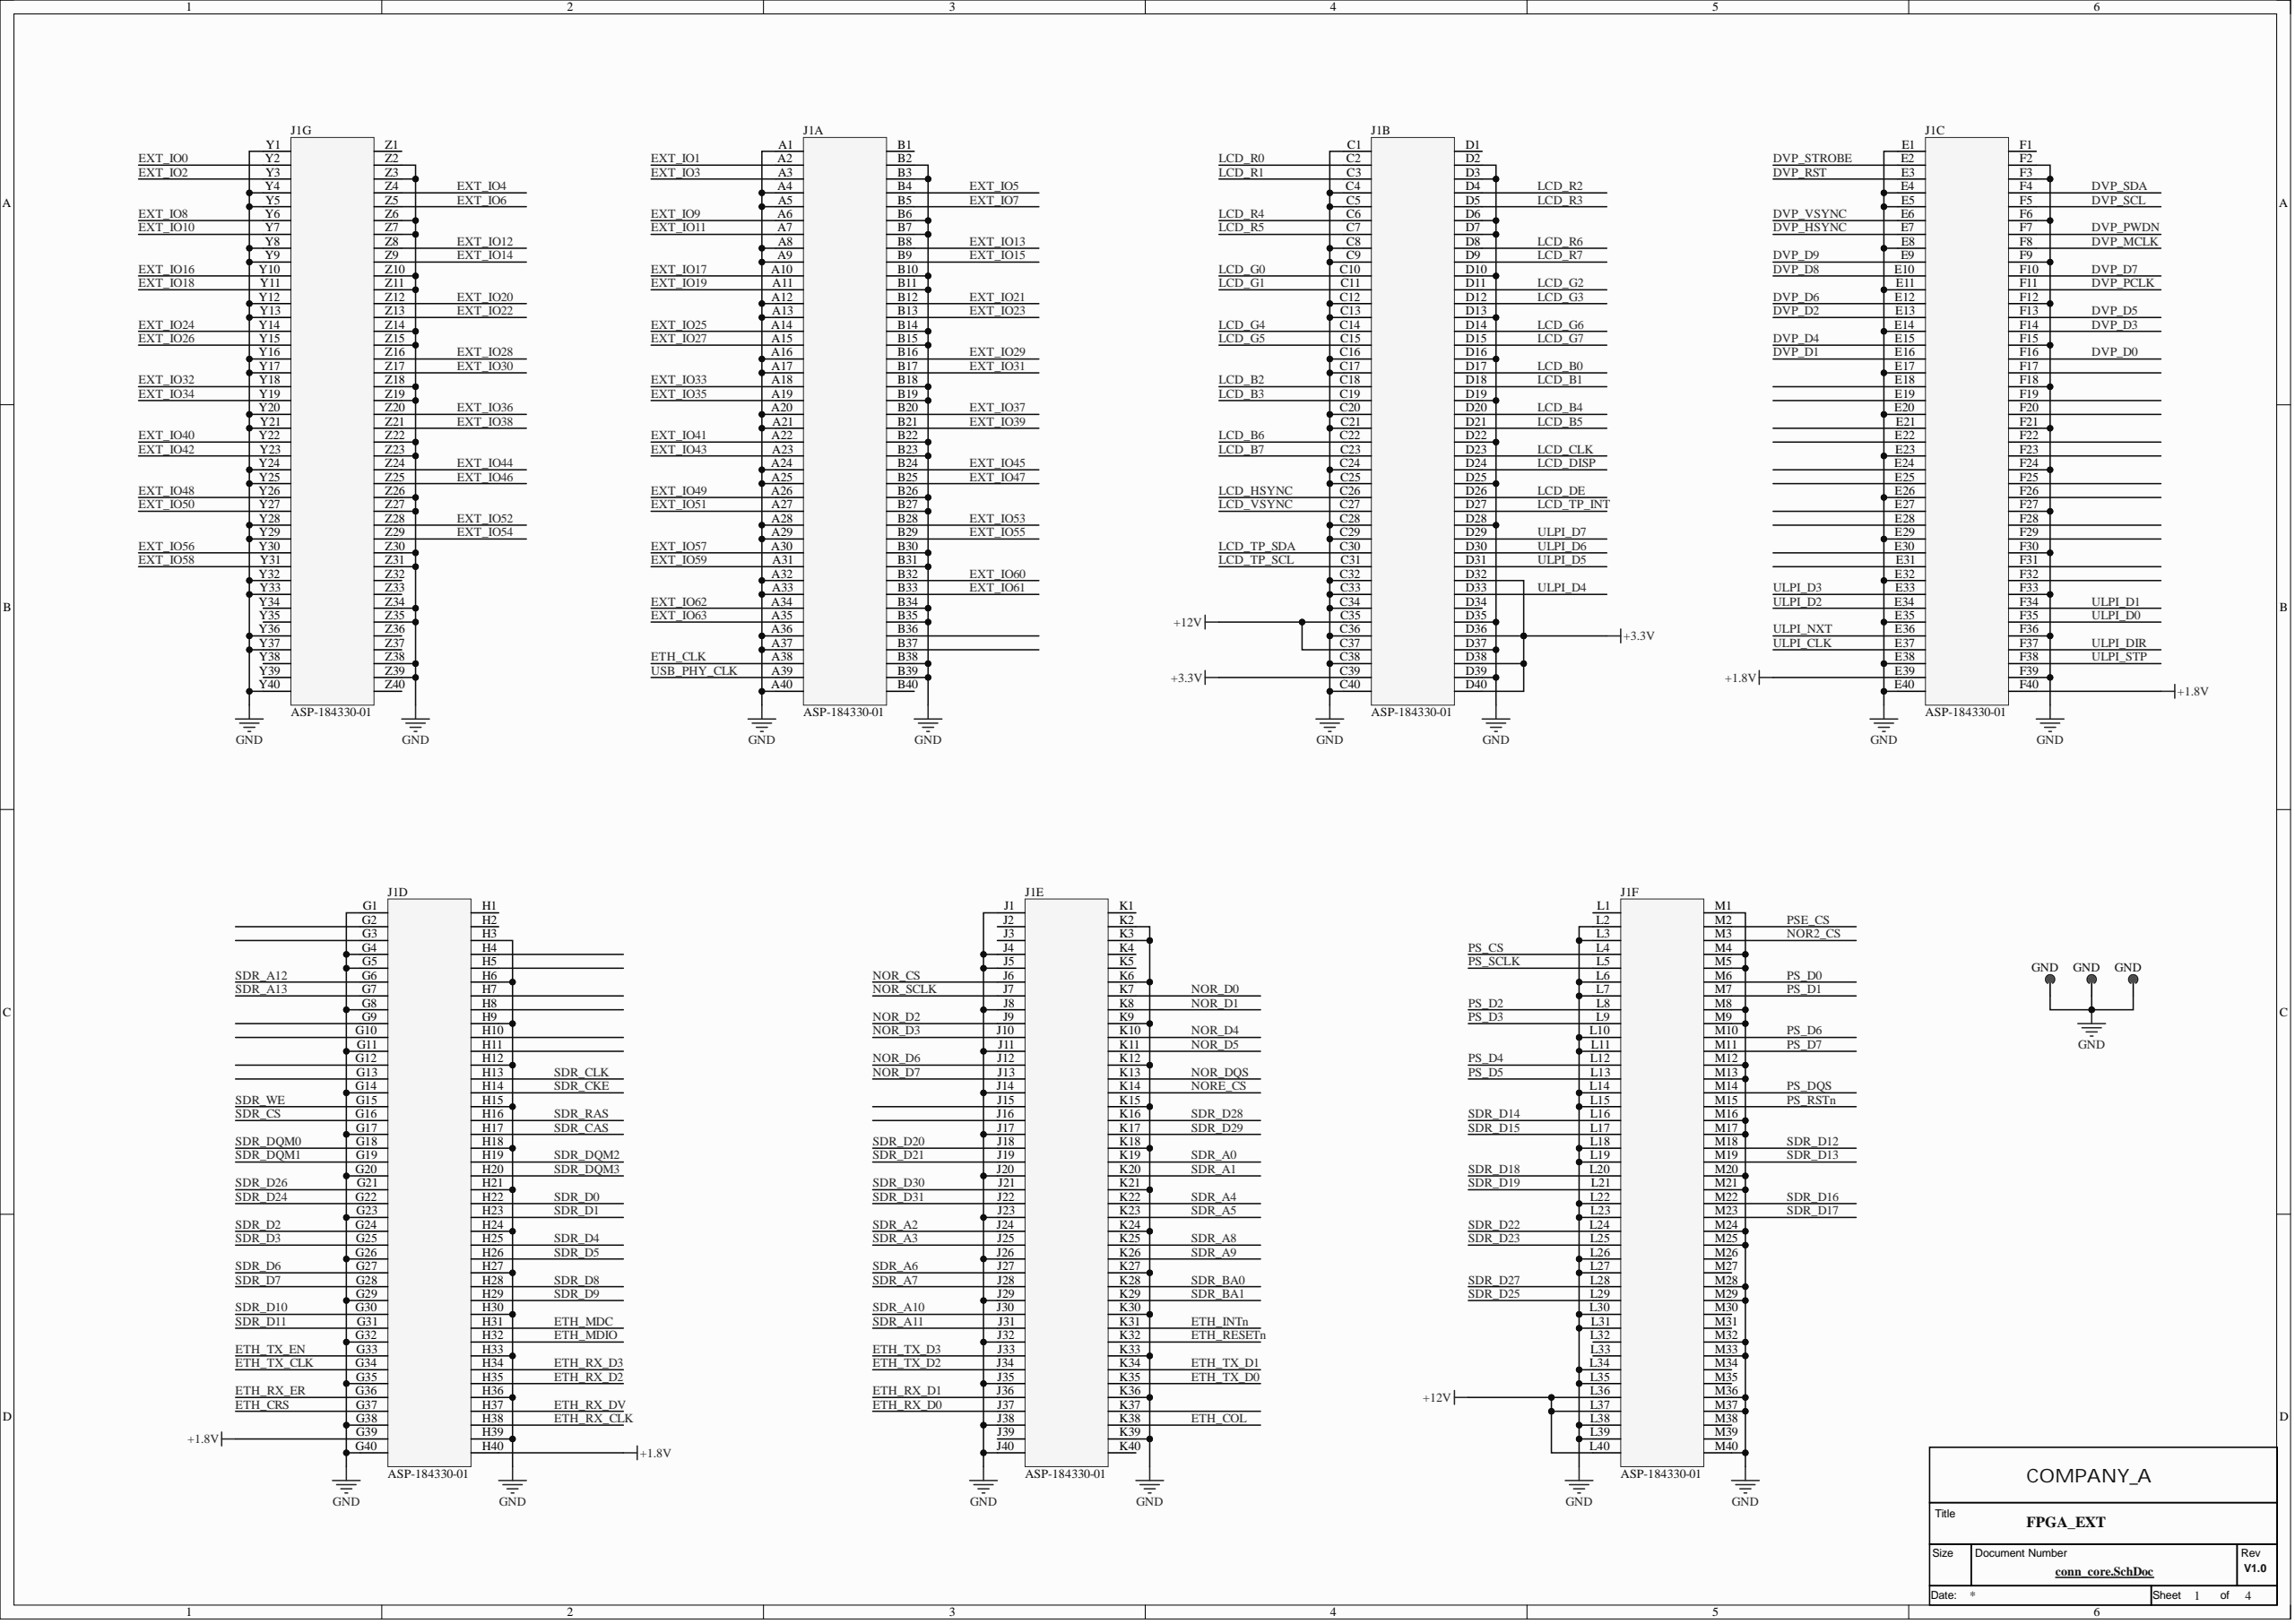Circuit board | Altium Designer | 234 parts | 308 nets | one sheet of the schematic
Parts on this sheet (reference | value | footprint):
J1 | ASP-184330-01 | ASP-184330-01_Bottom
J2 | FPC0.5-50P | FPC0.5-50P
J3 | FPC0.5-40P | FPC0.5-40P
J5 | CAM_DVP | FPC0.5-24P
Nets of these parts (net: part-pin ...):
USB_PHY_CLK: J1-A39
ULPI_STP: J1-F38
ULPI_NXT: J1-E36
ULPI_DIR: J1-F37
ULPI_D7: J1-D29
ULPI_D6: J1-D30
ULPI_D5: J1-D31
ULPI_D4: J1-D33
ULPI_D3: J1-E33
ULPI_D2: J1-E34
ULPI_D1: J1-F34
ULPI_D0: J1-F35
ULPI_CLK: J1-E37
SDR_WE: J1-G15
SDR_RAS: J1-H16
SDR_DQM3: J1-H20
SDR_DQM2: J1-H19
SDR_DQM1: J1-G19
SDR_DQM0: J1-G18
SDR_D31: J1-J22
SDR_D30: J1-J21
SDR_D29: J1-K17
SDR_D28: J1-K16
SDR_D27: J1-L28
SDR_D26: J1-G21
SDR_D25: J1-L29
SDR_D24: J1-G22
SDR_D23: J1-L25
SDR_D22: J1-L24
SDR_D21: J1-J19
SDR_D20: J1-J18
SDR_D19: J1-L21
SDR_D18: J1-L20
SDR_D17: J1-M23
SDR_D16: J1-M22
SDR_D15: J1-L17
SDR_D14: J1-L16
SDR_D13: J1-M19
SDR_D12: J1-M18
SDR_D11: J1-G31
SDR_D10: J1-G30
SDR_D9: J1-H29
SDR_D8: J1-H28
SDR_D7: J1-G28
SDR_D6: J1-G27
SDR_D5: J1-H26
SDR_D4: J1-H25
SDR_D3: J1-G25
SDR_D2: J1-G24
SDR_D1: J1-H23
SDR_D0: J1-H22
SDR_CS: J1-G16
SDR_CLK: J1-H13
SDR_CKE: J1-H14
SDR_CAS: J1-H17
SDR_BA1: J1-K29
SDR_BA0: J1-K28
SDR_A13: J1-G7
SDR_A12: J1-G6
SDR_A11: J1-J31
SDR_A10: J1-J30
SDR_A9: J1-K26
SDR_A8: J1-K25
SDR_A7: J1-J28
SDR_A6: J1-J27
SDR_A5: J1-K23
SDR_A4: J1-K22
SDR_A3: J1-J25
SDR_A2: J1-J24
SDR_A1: J1-K20
SDR_A0: J1-K19
PSE_CS: J1-M2
PS_SCLK: J1-L5
PS_RSTn: J1-M15
PS_DQS: J1-M14
PS_D7: J1-M11
PS_D6: J1-M10
PS_D5: J1-L13
PS_D4: J1-L12
PS_D3: J1-L9
PS_D2: J1-L8
PS_D1: J1-M7
PS_D0: J1-M6
PS_CS: J1-L4
NORE_CS: J1-K14
NOR_SCLK: J1-J7
NOR_DQS: J1-K13
NOR_D7: J1-J13
NOR_D6: J1-J12
NOR_D5: J1-K11
NOR_D4: J1-K10
NOR_D3: J1-J10
NOR_D2: J1-J9
NOR_D1: J1-K8
NOR_D0: J1-K7
NOR_CS: J1-J6
NOR2_CS: J1-M3
LCD_VSYNC: J1-C27
LCD_TP_SDA: J1-C30
LCD_TP_SCL: J1-C31
LCD_TP_INT: J1-D27
LCD_R7: J1-D9
LCD_R6: J1-D8
LCD_R5: J1-C7
LCD_R4: J1-C6
LCD_R3: J1-D5
LCD_R2: J1-D4
LCD_R1: J1-C3 J3-6
LCD_R0: J1-C2 J3-5
LCD_HSYNC: J1-C26
LCD_G7: J1-D15
LCD_G6: J1-D14
LCD_G5: J1-C15
LCD_G4: J1-C14
LCD_G3: J1-D12
LCD_G2: J1-D11
LCD_G1: J1-C11
LCD_G0: J1-C10
LCD_DISP: J1-D24
LCD_DE: J1-D26
LCD_CLK: J1-D23
LCD_B7: J1-C23
LCD_B6: J1-C22
LCD_B5: J1-D21
LCD_B4: J1-D20
LCD_B3: J1-C19
LCD_B2: J1-C18
LCD_B1: J1-D18
LCD_B0: J1-D17
GND: J1-A1 J1-A4 J1-A5 J1-A8 J1-A9 J1-A12 J1-A13 J1-A16 J1-A17 J1-A20 J1-A21 J1-A24 J1-A25 J1-A28 J1-A29 J1-A32 J1-A33 J1-A36 J1-A37 J1-A40 J1-B2 J1-B3 J1-B6 J1-B7 J1-B10 J1-B11 J1-B14 J1-B15 J1-B18 J1-B19 J1-B22 J1-B23 J1-B26 J1-B27 J1-B30 J1-B31 J1-B34 J1-B35 J1-B38 J1-B39 J1-C1 J1-C4 J1-C5 J1-C8 J1-C9 J1-C12 J1-C13 J1-C16 J1-C17 J1-C20 J1-C21 J1-C24 J1-C25 J1-C28 J1-C29 J1-C32 J1-C33 J1-C34 J1-C36 J1-C38 J1-C40 J1-D2 J1-D3 J1-D6 J1-D7 J1-D10 J1-D13 J1-D16 J1-D19 J1-D22 J1-D25 J1-D28 J1-D35 J1-D37 J1-D39 J1-E1 J1-E4 J1-E5 J1-E8 J1-E11 J1-E14 J1-E17 J1-E20 J1-E23 J1-E26 J1-E29 J1-E32 J1-E35 J1-E38 J1-E40 J1-F2 J1-F3 J1-F6 J1-F9 J1-F12 J1-F15 J1-F18 J1-F21 J1-F24 J1-F27 J1-F30 J1-F33 J1-F36 J1-F39 J1-G1 J1-G4 J1-G5 J1-G8 J1-G11 J1-G14 J1-G17 J1-G20 J1-G23 J1-G26 J1-G29 J1-G32 J1-G35 J1-G38 J1-G40 J1-H3 J1-H6 J1-H9 J1-H12 J1-H15 J1-H18 J1-H21 J1-H24 J1-H27 J1-H30 J1-H33 J1-H36 J1-H39 J1-J1 J1-J4 J1-J5 J1-J8 J1-J11 J1-J14 J1-J17 J1-J20 J1-J23 J1-J26 J1-J29 J1-J32 J1-J35 J1-J38 J1-J40 J1-K2 J1-K3 J1-K6 J1-K9 J1-K12 J1-K15 J1-K18 J1-K21 J1-K24 J1-K27 J1-K30 J1-K33 J1-K36 J1-K39 J1-L2 J1-L3 J1-L6 J1-L7 J1-L10 J1-L11 J1-L14 J1-L15 J1-L18 J1-L19 J1-L22 J1-L23 J1-L26 J1-L27 J1-L30 J1-L31 J1-L34 J1-L35 J1-L38 J1-L39 J1-M1 J1-M4 J1-M5 J1-M8 J1-M9 J1-M12 J1-M13 J1-M16 J1-M17 J1-M20 J1-M21 J1-M24 J1-M25 J1-M28 J1-M29 J1-M32 J1-M33 J1-M36 J1-M37 J1-M40 J1-Y1 J1-Y4 J1-Y5 J1-Y8 J1-Y9 J1-Y12 J1-Y13 J1-Y16 J1-Y17 J1-Y20 J1-Y21 J1-Y24 J1-Y25 J1-Y28 J1-Y29 J1-Y32 J1-Y33 J1-Y36 J1-Y37 J1-Y40 J1-Z2 J1-Z3 J1-Z6 J1-Z7 J1-Z10 J1-Z11 J1-Z14 J1-Z15 J1-Z18 J1-Z19 J1-Z22 J1-Z23 J1-Z26 J1-Z27 J1-Z30 J1-Z31 J1-Z34 J1-Z35 J1-Z38 J1-Z39 J2-5 J3-3 J5-2
EXT_IO63: J1-A35
EXT_IO62: J1-A34
EXT_IO61: J1-B33
EXT_IO60: J1-B32
EXT_IO59: J1-A31
EXT_IO58: J1-Y31
EXT_IO57: J1-A30
EXT_IO56: J1-Y30
EXT_IO55: J1-B29
EXT_IO54: J1-Z29
EXT_IO53: J1-B28
EXT_IO52: J1-Z28
EXT_IO51: J1-A27
EXT_IO50: J1-Y27
EXT_IO49: J1-A26
EXT_IO48: J1-Y26
EXT_IO47: J1-B25
EXT_IO46: J1-Z25
EXT_IO45: J1-B24
EXT_IO44: J1-Z24
EXT_IO43: J1-A23
EXT_IO42: J1-Y23
EXT_IO41: J1-A22
EXT_IO40: J1-Y22
EXT_IO39: J1-B21
EXT_IO38: J1-Z21
EXT_IO37: J1-B20
EXT_IO36: J1-Z20
EXT_IO35: J1-A19
EXT_IO34: J1-Y19
EXT_IO33: J1-A18
EXT_IO32: J1-Y18
EXT_IO31: J1-B17
EXT_IO30: J1-Z17
EXT_IO29: J1-B16
EXT_IO28: J1-Z16
EXT_IO27: J1-A15
EXT_IO26: J1-Y15
EXT_IO25: J1-A14
EXT_IO24: J1-Y14
EXT_IO23: J1-B13
EXT_IO22: J1-Z13
EXT_IO21: J1-B12
EXT_IO20: J1-Z12
EXT_IO19: J1-A11
EXT_IO18: J1-Y11
EXT_IO17: J1-A10
EXT_IO16: J1-Y10
EXT_IO15: J1-B9
EXT_IO14: J1-Z9
EXT_IO13: J1-B8
EXT_IO12: J1-Z8
EXT_IO11: J1-A7
EXT_IO10: J1-Y7
EXT_IO9: J1-A6
EXT_IO8: J1-Y6
EXT_IO7: J1-B5
EXT_IO6: J1-Z5
EXT_IO5: J1-B4
EXT_IO4: J1-Z4
EXT_IO3: J1-A3
EXT_IO2: J1-Y3
EXT_IO1: J1-A2
EXT_IO0: J1-Y2
ETH_TX_EN: J1-G33
ETH_TX_D3: J1-J33
ETH_TX_D2: J1-J34
ETH_TX_D1: J1-K34
ETH_TX_D0: J1-K35
ETH_TX_CLK: J1-G34
ETH_RX_ER: J1-G36
ETH_RX_DV: J1-H37
ETH_RX_D3: J1-H34
ETH_RX_D2: J1-H35
ETH_RX_D1: J1-J36
ETH_RX_D0: J1-J37
ETH_RX_CLK: J1-H38
ETH_RESETn: J1-K32
ETH_MDIO: J1-H32
ETH_MDC: J1-H31
ETH_INTn: J1-K31
ETH_CRS: J1-G37
ETH_COL: J1-K38
ETH_CLK: J1-A38
DVP_VSYNC: J1-E6
DVP_STROBE: J1-E2 J5-1
DVP_SDA: J1-F4 J5-3
DVP_SCL: J1-F5 J5-5
DVP_RST: J1-E3 J5-6
DVP_PWDN: J1-F7
DVP_PCLK: J1-F11
DVP_MCLK: J1-F8
DVP_HSYNC: J1-E7
DVP_D9: J1-E9
DVP_D8: J1-E10
DVP_D7: J1-F10
DVP_D6: J1-E12
DVP_D5: J1-F13
DVP_D4: J1-E15
DVP_D3: J1-F14
DVP_D2: J1-E13
DVP_D1: J1-E16
DVP_D0: J1-F16
+12V: J1-C35 J1-C37 J1-L36 J1-L37 J1-L40
+3.3V: J1-C39 J1-D32 J1-D36 J1-D38 J1-D40
+1.8V: J1-E39 J1-F40 J1-G39 J1-H40